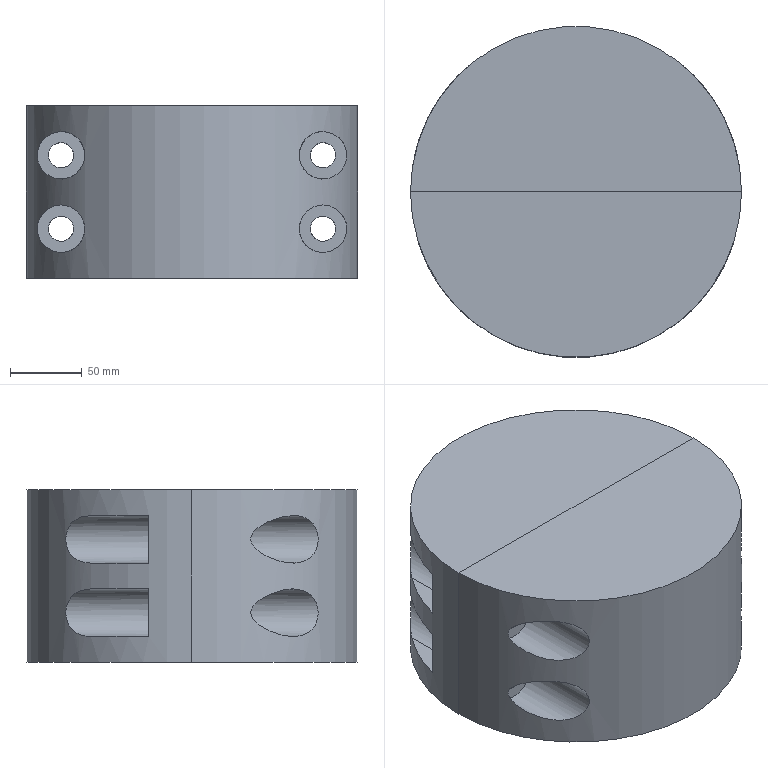Part | 2 solids | 40 faces | box 230 x 230 x 120 mm | volume 4635464 mm3 | plane 22 | cylinder 18 | commonest cylinder face diameters 33 x8 17.5 x4 21.5 x4 230 x2
STEP:
#1=CARTESIAN_POINT('',(-91.,-70.314,-69.));
#2=VERTEX_POINT('',#1);
#3=CARTESIAN_POINT('',(-96.354,-62.987,-69.619));
#4=CARTESIAN_POINT('',(-91.082,-70.404,-68.695));
#5=CARTESIAN_POINT('',(-85.319,-77.28,-69.6));
#6=CARTESIAN_POINT('',(-79.311,-83.397,-73.048));
#7=CARTESIAN_POINT('',(-75.355,-86.883,-78.919));
#8=CARTESIAN_POINT('',(-74.295,-87.779,-84.937));
#9=CARTESIAN_POINT('',(-74.785,-87.366,-89.518));
#10=CARTESIAN_POINT('',(-76.421,-85.949,-93.603));
#11=CARTESIAN_POINT('',(-79.627,-83.033,-97.936));
#12=CARTESIAN_POINT('',(-84.578,-78.089,-101.141));
#13=CARTESIAN_POINT('',(-90.444,-71.222,-102.304));
#14=CARTESIAN_POINT('',(-95.772,-63.869,-101.569));
#15=CARTESIAN_POINT('',(-99.558,-57.683,-99.78));
#16=CARTESIAN_POINT('',(-102.236,-52.713,-97.676));
#17=CARTESIAN_POINT('',(-104.052,-49.025,-95.718));
#18=CARTESIAN_POINT('',(-105.632,-45.513,-93.32));
#19=CARTESIAN_POINT('',(-106.715,-42.878,-90.795));
#20=CARTESIAN_POINT('',(-107.32,-41.324,-88.221));
#21=CARTESIAN_POINT('',(-107.546,-40.729,-86.006));
#22=CARTESIAN_POINT('',(-107.453,-40.976,-83.706));
#23=CARTESIAN_POINT('',(-106.959,-42.26,-80.962));
#24=CARTESIAN_POINT('',(-105.94,-44.789,-78.271));
#25=CARTESIAN_POINT('',(-104.42,-48.235,-75.768));
#26=CARTESIAN_POINT('',(-102.668,-51.865,-73.736));
#27=CARTESIAN_POINT('',(-100.044,-56.834,-71.521));
#28=CARTESIAN_POINT('',(-96.354,-62.987,-69.619));
#29=CARTESIAN_POINT('',(-91.082,-70.404,-68.695));
#30=CARTESIAN_POINT('',(-85.319,-77.28,-69.6));
#31=B_SPLINE_CURVE_WITH_KNOTS('',3,(#3,#4,#5,#6,#7,#8,#9,#10,#11,#12,#13,#14,#15,#16,#17,#18,#19,#20,#21,#22,#23,#24,#25,#26,#27,#28,#29,#30),.UNSPECIFIED.,.T.,.F.,(1,1,1,1,1,1,1,1,1,1,1,1,1,1,1,1,1,1,1,1,1,1,1,1,1,1,1,1,1,1,1,1),(-0.02241,-0.01793,-0.008966,0.,0.008966,0.01793,0.0269,0.03138,0.03586,0.04035,0.04483,0.05379,0.06276,0.07173,0.08069,0.08517,0.08966,0.09414,0.09862,0.1009,0.1031,0.1053,0.1076,0.1121,0.1166,0.121,0.1255,0.1345,0.1435,0.1524,0.1614,0.1703),.UNSPECIFIED.);
#32=EDGE_CURVE('',#2,#2,#31,.T.);
#33=ORIENTED_EDGE('',*,*,#32,.F.);
#34=EDGE_LOOP('',(#33));
#35=FACE_BOUND('',#34,.T.);
#36=CARTESIAN_POINT('',(-107.5,-30.,-85.5));
#37=VERTEX_POINT('',#36);
#38=CARTESIAN_POINT('',(-91.,-30.,-85.5));
#39=DIRECTION('',(0.,-1.,0.));
#40=DIRECTION('',(-1.,0.,0.));
#41=AXIS2_PLACEMENT_3D('',#38,#39,#40);
#42=CIRCLE('',#41,16.5);
#43=EDGE_CURVE('',#37,#37,#42,.T.);
#44=ORIENTED_EDGE('',*,*,#43,.F.);
#45=EDGE_LOOP('',(#44));
#46=FACE_BOUND('',#45,.T.);
#47=CARTESIAN_POINT('',(-91.,-120.,-85.5));
#48=DIRECTION('',(0.,1.,0.));
#49=DIRECTION('',(0.,0.,1.));
#50=AXIS2_PLACEMENT_3D('',#47,#48,#49);
#51=CYLINDRICAL_SURFACE('',#50,16.5);
#52=ADVANCED_FACE('',(#35,#46),#51,.F.);
#53=CARTESIAN_POINT('',(-91.,-30.,-76.75));
#54=VERTEX_POINT('',#53);
#55=CARTESIAN_POINT('',(-91.,-30.,-85.5));
#56=DIRECTION('',(0.,-1.,0.));
#57=DIRECTION('',(0.,0.,1.));
#58=AXIS2_PLACEMENT_3D('',#55,#56,#57);
#59=CIRCLE('',#58,8.75);
#60=EDGE_CURVE('',#54,#54,#59,.T.);
#61=ORIENTED_EDGE('',*,*,#60,.F.);
#62=EDGE_LOOP('',(#61));
#63=FACE_BOUND('',#62,.T.);
#64=ORIENTED_EDGE('',*,*,#43,.T.);
#65=EDGE_LOOP('',(#64));
#66=FACE_BOUND('',#65,.T.);
#67=CARTESIAN_POINT('',(-91.,-30.,-85.5));
#68=DIRECTION('',(0.,1.,0.));
#69=DIRECTION('',(0.,0.,1.));
#70=AXIS2_PLACEMENT_3D('',#67,#68,#69);
#71=PLANE('',#70);
#72=ADVANCED_FACE('',(#63,#66),#71,.F.);
#73=CARTESIAN_POINT('',(-99.75,0.,-85.5));
#74=VERTEX_POINT('',#73);
#75=CARTESIAN_POINT('',(-91.,0.,-85.5));
#76=DIRECTION('',(0.,1.,0.));
#77=DIRECTION('',(-1.,0.,0.));
#78=AXIS2_PLACEMENT_3D('',#75,#76,#77);
#79=CIRCLE('',#78,8.75);
#80=EDGE_CURVE('',#74,#74,#79,.F.);
#81=ORIENTED_EDGE('',*,*,#80,.F.);
#82=EDGE_LOOP('',(#81));
#83=FACE_BOUND('',#82,.T.);
#84=ORIENTED_EDGE('',*,*,#60,.T.);
#85=EDGE_LOOP('',(#84));
#86=FACE_BOUND('',#85,.T.);
#87=CARTESIAN_POINT('',(-91.,-120.,-85.5));
#88=DIRECTION('',(0.,1.,0.));
#89=DIRECTION('',(0.,0.,1.));
#90=AXIS2_PLACEMENT_3D('',#87,#88,#89);
#91=CYLINDRICAL_SURFACE('',#90,8.75);
#92=ADVANCED_FACE('',(#83,#86),#91,.F.);
#93=CARTESIAN_POINT('',(-91.,-30.,-43.25));
#94=VERTEX_POINT('',#93);
#95=CARTESIAN_POINT('',(-91.,-30.,-34.5));
#96=DIRECTION('',(0.,1.,0.));
#97=DIRECTION('',(0.,0.,-1.));
#98=AXIS2_PLACEMENT_3D('',#95,#96,#97);
#99=CIRCLE('',#98,8.75);
#100=EDGE_CURVE('',#94,#94,#99,.F.);
#101=ORIENTED_EDGE('',*,*,#100,.T.);
#102=EDGE_LOOP('',(#101));
#103=FACE_BOUND('',#102,.T.);
#104=CARTESIAN_POINT('',(-99.75,0.,-34.5));
#105=VERTEX_POINT('',#104);
#106=CARTESIAN_POINT('',(-91.,0.,-34.5));
#107=DIRECTION('',(0.,-1.,0.));
#108=DIRECTION('',(-1.,0.,0.));
#109=AXIS2_PLACEMENT_3D('',#106,#107,#108);
#110=CIRCLE('',#109,8.75);
#111=EDGE_CURVE('',#105,#105,#110,.T.);
#112=ORIENTED_EDGE('',*,*,#111,.F.);
#113=EDGE_LOOP('',(#112));
#114=FACE_BOUND('',#113,.T.);
#115=CARTESIAN_POINT('',(-91.,-120.,-34.5));
#116=DIRECTION('',(0.,1.,0.));
#117=DIRECTION('',(0.,0.,1.));
#118=AXIS2_PLACEMENT_3D('',#115,#116,#117);
#119=CYLINDRICAL_SURFACE('',#118,8.75);
#120=ADVANCED_FACE('',(#103,#114),#119,.F.);
#121=ORIENTED_EDGE('',*,*,#100,.F.);
#122=EDGE_LOOP('',(#121));
#123=FACE_BOUND('',#122,.T.);
#124=CARTESIAN_POINT('',(-107.5,-30.,-34.5));
#125=VERTEX_POINT('',#124);
#126=CARTESIAN_POINT('',(-91.,-30.,-34.5));
#127=DIRECTION('',(0.,1.,0.));
#128=DIRECTION('',(-1.,0.,0.));
#129=AXIS2_PLACEMENT_3D('',#126,#127,#128);
#130=CIRCLE('',#129,16.5);
#131=EDGE_CURVE('',#125,#125,#130,.T.);
#132=ORIENTED_EDGE('',*,*,#131,.F.);
#133=EDGE_LOOP('',(#132));
#134=FACE_BOUND('',#133,.T.);
#135=CARTESIAN_POINT('',(-91.,-30.,-34.5));
#136=DIRECTION('',(0.,-1.,0.));
#137=DIRECTION('',(0.,0.,-1.));
#138=AXIS2_PLACEMENT_3D('',#135,#136,#137);
#139=PLANE('',#138);
#140=ADVANCED_FACE('',(#123,#134),#139,.T.);
#141=CARTESIAN_POINT('',(-91.,-70.314,-18.));
#142=VERTEX_POINT('',#141);
#143=CARTESIAN_POINT('',(-85.296,-77.307,-18.605));
#144=CARTESIAN_POINT('',(-91.099,-70.38,-17.698));
#145=CARTESIAN_POINT('',(-95.44,-64.276,-18.453));
#146=CARTESIAN_POINT('',(-98.544,-59.334,-19.753));
#147=CARTESIAN_POINT('',(-100.712,-55.572,-21.081));
#148=CARTESIAN_POINT('',(-102.66,-51.88,-22.731));
#149=CARTESIAN_POINT('',(-104.409,-48.258,-24.752));
#150=CARTESIAN_POINT('',(-105.937,-44.797,-27.266));
#151=CARTESIAN_POINT('',(-106.953,-42.277,-29.937));
#152=CARTESIAN_POINT('',(-107.452,-40.979,-32.694));
#153=CARTESIAN_POINT('',(-107.547,-40.727,-34.996));
#154=CARTESIAN_POINT('',(-107.319,-41.327,-37.229));
#155=CARTESIAN_POINT('',(-106.714,-42.88,-39.795));
#156=CARTESIAN_POINT('',(-105.63,-45.518,-42.326));
#157=CARTESIAN_POINT('',(-104.046,-49.037,-44.723));
#158=CARTESIAN_POINT('',(-102.253,-52.679,-46.66));
#159=CARTESIAN_POINT('',(-99.557,-57.686,-48.784));
#160=CARTESIAN_POINT('',(-95.779,-63.857,-50.565));
#161=CARTESIAN_POINT('',(-90.458,-71.205,-51.304));
#162=CARTESIAN_POINT('',(-84.59,-78.077,-50.146));
#163=CARTESIAN_POINT('',(-79.635,-83.026,-46.942));
#164=CARTESIAN_POINT('',(-76.43,-85.941,-42.618));
#165=CARTESIAN_POINT('',(-74.794,-87.359,-38.545));
#166=CARTESIAN_POINT('',(-74.294,-87.779,-33.985));
#167=CARTESIAN_POINT('',(-75.338,-86.898,-27.95));
#168=CARTESIAN_POINT('',(-79.304,-83.403,-22.055));
#169=CARTESIAN_POINT('',(-85.296,-77.307,-18.605));
#170=CARTESIAN_POINT('',(-91.099,-70.38,-17.698));
#171=CARTESIAN_POINT('',(-95.44,-64.276,-18.453));
#172=B_SPLINE_CURVE_WITH_KNOTS('',3,(#143,#144,#145,#146,#147,#148,#149,#150,#151,#152,#153,#154,#155,#156,#157,#158,#159,#160,#161,#162,#163,#164,#165,#166,#167,#168,#169,#170,#171),.UNSPECIFIED.,.T.,.F.,(1,1,1,1,1,1,1,1,1,1,1,1,1,1,1,1,1,1,1,1,1,1,1,1,1,1,1,1,1,1,1,1,1),(-0.02687,-0.01791,-0.008956,0.,0.008956,0.01343,0.01791,0.02239,0.02687,0.03135,0.03583,0.03806,0.0403,0.04254,0.04478,0.04926,0.05374,0.05822,0.06269,0.07165,0.08061,0.08956,0.09852,0.103,0.1075,0.112,0.1164,0.1254,0.1343,0.1433,0.1523,0.1567,0.1612),.UNSPECIFIED.);
#173=EDGE_CURVE('',#142,#142,#172,.F.);
#174=ORIENTED_EDGE('',*,*,#173,.F.);
#175=EDGE_LOOP('',(#174));
#176=FACE_BOUND('',#175,.T.);
#177=ORIENTED_EDGE('',*,*,#131,.T.);
#178=EDGE_LOOP('',(#177));
#179=FACE_BOUND('',#178,.T.);
#180=CARTESIAN_POINT('',(-91.,-120.,-34.5));
#181=DIRECTION('',(0.,1.,0.));
#182=DIRECTION('',(0.,0.,1.));
#183=AXIS2_PLACEMENT_3D('',#180,#181,#182);
#184=CYLINDRICAL_SURFACE('',#183,16.5);
#185=ADVANCED_FACE('',(#176,#179),#184,.F.);
#186=CARTESIAN_POINT('',(91.,-30.,-43.25));
#187=VERTEX_POINT('',#186);
#188=CARTESIAN_POINT('',(91.,-30.,-34.5));
#189=DIRECTION('',(0.,-1.,0.));
#190=DIRECTION('',(0.,0.,-1.));
#191=AXIS2_PLACEMENT_3D('',#188,#189,#190);
#192=CIRCLE('',#191,8.75);
#193=EDGE_CURVE('',#187,#187,#192,.T.);
#194=ORIENTED_EDGE('',*,*,#193,.F.);
#195=EDGE_LOOP('',(#194));
#196=FACE_BOUND('',#195,.T.);
#197=CARTESIAN_POINT('',(107.5,-30.,-34.5));
#198=VERTEX_POINT('',#197);
#199=CARTESIAN_POINT('',(91.,-30.,-34.5));
#200=DIRECTION('',(0.,-1.,0.));
#201=DIRECTION('',(1.,0.,0.));
#202=AXIS2_PLACEMENT_3D('',#199,#200,#201);
#203=CIRCLE('',#202,16.5);
#204=EDGE_CURVE('',#198,#198,#203,.F.);
#205=ORIENTED_EDGE('',*,*,#204,.F.);
#206=EDGE_LOOP('',(#205));
#207=FACE_BOUND('',#206,.T.);
#208=CARTESIAN_POINT('',(91.,-30.,-34.5));
#209=DIRECTION('',(0.,-1.,0.));
#210=DIRECTION('',(0.,0.,-1.));
#211=AXIS2_PLACEMENT_3D('',#208,#209,#210);
#212=PLANE('',#211);
#213=ADVANCED_FACE('',(#196,#207),#212,.T.);
#214=CARTESIAN_POINT('',(91.,-30.,-76.75));
#215=VERTEX_POINT('',#214);
#216=CARTESIAN_POINT('',(91.,-30.,-85.5));
#217=DIRECTION('',(0.,1.,0.));
#218=DIRECTION('',(0.,0.,1.));
#219=AXIS2_PLACEMENT_3D('',#216,#217,#218);
#220=CIRCLE('',#219,8.75);
#221=EDGE_CURVE('',#215,#215,#220,.F.);
#222=ORIENTED_EDGE('',*,*,#221,.F.);
#223=EDGE_LOOP('',(#222));
#224=FACE_BOUND('',#223,.T.);
#225=CARTESIAN_POINT('',(107.5,-30.,-85.5));
#226=VERTEX_POINT('',#225);
#227=CARTESIAN_POINT('',(91.,-30.,-85.5));
#228=DIRECTION('',(0.,1.,0.));
#229=DIRECTION('',(1.,0.,0.));
#230=AXIS2_PLACEMENT_3D('',#227,#228,#229);
#231=CIRCLE('',#230,16.5);
#232=EDGE_CURVE('',#226,#226,#231,.F.);
#233=ORIENTED_EDGE('',*,*,#232,.T.);
#234=EDGE_LOOP('',(#233));
#235=FACE_BOUND('',#234,.T.);
#236=CARTESIAN_POINT('',(91.,-30.,-85.5));
#237=DIRECTION('',(0.,1.,0.));
#238=DIRECTION('',(0.,0.,1.));
#239=AXIS2_PLACEMENT_3D('',#236,#237,#238);
#240=PLANE('',#239);
#241=ADVANCED_FACE('',(#224,#235),#240,.F.);
#242=ORIENTED_EDGE('',*,*,#193,.T.);
#243=EDGE_LOOP('',(#242));
#244=FACE_BOUND('',#243,.T.);
#245=CARTESIAN_POINT('',(99.75,0.,-34.5));
#246=VERTEX_POINT('',#245);
#247=CARTESIAN_POINT('',(91.,0.,-34.5));
#248=DIRECTION('',(0.,1.,0.));
#249=DIRECTION('',(1.,0.,0.));
#250=AXIS2_PLACEMENT_3D('',#247,#248,#249);
#251=CIRCLE('',#250,8.75);
#252=EDGE_CURVE('',#246,#246,#251,.T.);
#253=ORIENTED_EDGE('',*,*,#252,.T.);
#254=EDGE_LOOP('',(#253));
#255=FACE_BOUND('',#254,.T.);
#256=CARTESIAN_POINT('',(91.,-120.,-34.5));
#257=DIRECTION('',(0.,1.,0.));
#258=DIRECTION('',(0.,0.,1.));
#259=AXIS2_PLACEMENT_3D('',#256,#257,#258);
#260=CYLINDRICAL_SURFACE('',#259,8.75);
#261=ADVANCED_FACE('',(#244,#255),#260,.F.);
#262=CARTESIAN_POINT('',(99.75,0.,-85.5));
#263=VERTEX_POINT('',#262);
#264=CARTESIAN_POINT('',(91.,0.,-85.5));
#265=DIRECTION('',(0.,-1.,0.));
#266=DIRECTION('',(1.,0.,0.));
#267=AXIS2_PLACEMENT_3D('',#264,#265,#266);
#268=CIRCLE('',#267,8.75);
#269=EDGE_CURVE('',#263,#263,#268,.T.);
#270=ORIENTED_EDGE('',*,*,#269,.F.);
#271=EDGE_LOOP('',(#270));
#272=FACE_BOUND('',#271,.T.);
#273=ORIENTED_EDGE('',*,*,#221,.T.);
#274=EDGE_LOOP('',(#273));
#275=FACE_BOUND('',#274,.T.);
#276=CARTESIAN_POINT('',(91.,-120.,-85.5));
#277=DIRECTION('',(0.,1.,0.));
#278=DIRECTION('',(0.,0.,1.));
#279=AXIS2_PLACEMENT_3D('',#276,#277,#278);
#280=CYLINDRICAL_SURFACE('',#279,8.75);
#281=ADVANCED_FACE('',(#272,#275),#280,.F.);
#282=CARTESIAN_POINT('',(91.,-70.314,-18.));
#283=VERTEX_POINT('',#282);
#284=CARTESIAN_POINT('',(85.296,-77.307,-18.605));
#285=CARTESIAN_POINT('',(91.099,-70.38,-17.698));
#286=CARTESIAN_POINT('',(95.44,-64.276,-18.453));
#287=CARTESIAN_POINT('',(98.544,-59.334,-19.753));
#288=CARTESIAN_POINT('',(100.712,-55.572,-21.081));
#289=CARTESIAN_POINT('',(102.66,-51.88,-22.731));
#290=CARTESIAN_POINT('',(104.409,-48.258,-24.752));
#291=CARTESIAN_POINT('',(105.937,-44.797,-27.266));
#292=CARTESIAN_POINT('',(106.953,-42.277,-29.937));
#293=CARTESIAN_POINT('',(107.452,-40.979,-32.694));
#294=CARTESIAN_POINT('',(107.547,-40.727,-34.996));
#295=CARTESIAN_POINT('',(107.319,-41.327,-37.229));
#296=CARTESIAN_POINT('',(106.714,-42.88,-39.795));
#297=CARTESIAN_POINT('',(105.63,-45.518,-42.326));
#298=CARTESIAN_POINT('',(104.046,-49.037,-44.723));
#299=CARTESIAN_POINT('',(102.253,-52.679,-46.66));
#300=CARTESIAN_POINT('',(99.557,-57.686,-48.784));
#301=CARTESIAN_POINT('',(95.779,-63.857,-50.565));
#302=CARTESIAN_POINT('',(90.458,-71.205,-51.304));
#303=CARTESIAN_POINT('',(84.59,-78.077,-50.146));
#304=CARTESIAN_POINT('',(79.635,-83.026,-46.942));
#305=CARTESIAN_POINT('',(76.43,-85.941,-42.618));
#306=CARTESIAN_POINT('',(74.794,-87.359,-38.545));
#307=CARTESIAN_POINT('',(74.294,-87.779,-33.985));
#308=CARTESIAN_POINT('',(75.338,-86.898,-27.95));
#309=CARTESIAN_POINT('',(79.304,-83.403,-22.055));
#310=CARTESIAN_POINT('',(85.296,-77.307,-18.605));
#311=CARTESIAN_POINT('',(91.099,-70.38,-17.698));
#312=CARTESIAN_POINT('',(95.44,-64.276,-18.453));
#313=B_SPLINE_CURVE_WITH_KNOTS('',3,(#284,#285,#286,#287,#288,#289,#290,#291,#292,#293,#294,#295,#296,#297,#298,#299,#300,#301,#302,#303,#304,#305,#306,#307,#308,#309,#310,#311,#312),.UNSPECIFIED.,.T.,.F.,(1,1,1,1,1,1,1,1,1,1,1,1,1,1,1,1,1,1,1,1,1,1,1,1,1,1,1,1,1,1,1,1,1),(-0.02687,-0.01791,-0.008956,0.,0.008956,0.01343,0.01791,0.02239,0.02687,0.03135,0.03583,0.03806,0.0403,0.04254,0.04478,0.04926,0.05374,0.05822,0.06269,0.07165,0.08061,0.08956,0.09852,0.103,0.1075,0.112,0.1164,0.1254,0.1343,0.1433,0.1523,0.1567,0.1612),.UNSPECIFIED.);
#314=EDGE_CURVE('',#283,#283,#313,.T.);
#315=ORIENTED_EDGE('',*,*,#314,.F.);
#316=EDGE_LOOP('',(#315));
#317=FACE_BOUND('',#316,.T.);
#318=ORIENTED_EDGE('',*,*,#204,.T.);
#319=EDGE_LOOP('',(#318));
#320=FACE_BOUND('',#319,.T.);
#321=CARTESIAN_POINT('',(91.,-120.,-34.5));
#322=DIRECTION('',(0.,1.,0.));
#323=DIRECTION('',(0.,0.,1.));
#324=AXIS2_PLACEMENT_3D('',#321,#322,#323);
#325=CYLINDRICAL_SURFACE('',#324,16.5);
#326=ADVANCED_FACE('',(#317,#320),#325,.F.);
#327=CARTESIAN_POINT('',(-115.,0.,-120.));
#328=VERTEX_POINT('',#327);
#329=CARTESIAN_POINT('',(115.,0.,-120.));
#330=VERTEX_POINT('',#329);
#331=CARTESIAN_POINT('',(0.,0.,-120.));
#332=DIRECTION('',(0.,0.,1.));
#333=DIRECTION('',(1.,0.,0.));
#334=AXIS2_PLACEMENT_3D('',#331,#332,#333);
#335=CIRCLE('',#334,115.);
#336=EDGE_CURVE('',#328,#330,#335,.T.);
#337=ORIENTED_EDGE('',*,*,#336,.F.);
#338=CARTESIAN_POINT('',(115.,0.,-120.));
#339=DIRECTION('',(-1.,0.,0.));
#340=VECTOR('',#339,1000.);
#341=LINE('',#338,#340);
#342=EDGE_CURVE('',#330,#328,#341,.T.);
#343=ORIENTED_EDGE('',*,*,#342,.F.);
#344=EDGE_LOOP('',(#337,#343));
#345=FACE_BOUND('',#344,.T.);
#346=CARTESIAN_POINT('',(0.,0.,-120.));
#347=DIRECTION('',(0.,0.,1.));
#348=DIRECTION('',(1.,0.,0.));
#349=AXIS2_PLACEMENT_3D('',#346,#347,#348);
#350=PLANE('',#349);
#351=ADVANCED_FACE('',(#345),#350,.F.);
#352=ORIENTED_EDGE('',*,*,#80,.T.);
#353=EDGE_LOOP('',(#352));
#354=FACE_BOUND('',#353,.T.);
#355=ORIENTED_EDGE('',*,*,#111,.T.);
#356=EDGE_LOOP('',(#355));
#357=FACE_BOUND('',#356,.T.);
#358=ORIENTED_EDGE('',*,*,#269,.T.);
#359=EDGE_LOOP('',(#358));
#360=FACE_BOUND('',#359,.T.);
#361=CARTESIAN_POINT('',(115.,0.,0.));
#362=VERTEX_POINT('',#361);
#363=CARTESIAN_POINT('',(-115.,0.,0.));
#364=VERTEX_POINT('',#363);
#365=CARTESIAN_POINT('',(115.,0.,0.));
#366=DIRECTION('',(-1.,0.,0.));
#367=VECTOR('',#366,1000.);
#368=LINE('',#365,#367);
#369=EDGE_CURVE('',#362,#364,#368,.T.);
#370=ORIENTED_EDGE('',*,*,#369,.F.);
#371=CARTESIAN_POINT('',(115.,0.,-120.));
#372=DIRECTION('',(0.,0.,1.));
#373=VECTOR('',#372,1000.);
#374=LINE('',#371,#373);
#375=EDGE_CURVE('',#330,#362,#374,.T.);
#376=ORIENTED_EDGE('',*,*,#375,.F.);
#377=ORIENTED_EDGE('',*,*,#342,.T.);
#378=CARTESIAN_POINT('',(-115.,0.,-120.));
#379=DIRECTION('',(0.,0.,1.));
#380=VECTOR('',#379,1000.);
#381=LINE('',#378,#380);
#382=EDGE_CURVE('',#364,#328,#381,.F.);
#383=ORIENTED_EDGE('',*,*,#382,.F.);
#384=EDGE_LOOP('',(#370,#376,#377,#383));
#385=FACE_BOUND('',#384,.T.);
#386=ORIENTED_EDGE('',*,*,#252,.F.);
#387=EDGE_LOOP('',(#386));
#388=FACE_BOUND('',#387,.T.);
#389=CARTESIAN_POINT('',(115.,0.,-120.));
#390=DIRECTION('',(0.,1.,0.));
#391=DIRECTION('',(0.,0.,1.));
#392=AXIS2_PLACEMENT_3D('',#389,#390,#391);
#393=PLANE('',#392);
#394=ADVANCED_FACE('',(#354,#357,#360,#385,#388),#393,.T.);
#395=CARTESIAN_POINT('',(0.,0.,0.));
#396=DIRECTION('',(0.,0.,1.));
#397=DIRECTION('',(1.,0.,0.));
#398=AXIS2_PLACEMENT_3D('',#395,#396,#397);
#399=CIRCLE('',#398,115.);
#400=EDGE_CURVE('',#364,#362,#399,.T.);
#401=ORIENTED_EDGE('',*,*,#400,.T.);
#402=ORIENTED_EDGE('',*,*,#369,.T.);
#403=EDGE_LOOP('',(#401,#402));
#404=FACE_BOUND('',#403,.T.);
#405=CARTESIAN_POINT('',(0.,0.,0.));
#406=DIRECTION('',(0.,0.,1.));
#407=DIRECTION('',(1.,0.,0.));
#408=AXIS2_PLACEMENT_3D('',#405,#406,#407);
#409=PLANE('',#408);
#410=ADVANCED_FACE('',(#404),#409,.T.);
#411=CARTESIAN_POINT('',(91.,-70.314,-69.));
#412=VERTEX_POINT('',#411);
#413=CARTESIAN_POINT('',(96.354,-62.987,-69.619));
#414=CARTESIAN_POINT('',(91.082,-70.404,-68.695));
#415=CARTESIAN_POINT('',(85.319,-77.28,-69.6));
#416=CARTESIAN_POINT('',(79.311,-83.397,-73.048));
#417=CARTESIAN_POINT('',(75.355,-86.883,-78.919));
#418=CARTESIAN_POINT('',(74.295,-87.779,-84.937));
#419=CARTESIAN_POINT('',(74.785,-87.366,-89.518));
#420=CARTESIAN_POINT('',(76.421,-85.949,-93.603));
#421=CARTESIAN_POINT('',(79.627,-83.033,-97.936));
#422=CARTESIAN_POINT('',(84.578,-78.089,-101.141));
#423=CARTESIAN_POINT('',(90.444,-71.222,-102.304));
#424=CARTESIAN_POINT('',(95.772,-63.869,-101.569));
#425=CARTESIAN_POINT('',(99.558,-57.683,-99.78));
#426=CARTESIAN_POINT('',(102.236,-52.713,-97.676));
#427=CARTESIAN_POINT('',(104.052,-49.025,-95.718));
#428=CARTESIAN_POINT('',(105.632,-45.513,-93.32));
#429=CARTESIAN_POINT('',(106.715,-42.878,-90.795));
#430=CARTESIAN_POINT('',(107.32,-41.324,-88.221));
#431=CARTESIAN_POINT('',(107.546,-40.729,-86.006));
#432=CARTESIAN_POINT('',(107.453,-40.976,-83.706));
#433=CARTESIAN_POINT('',(106.959,-42.26,-80.962));
#434=CARTESIAN_POINT('',(105.94,-44.789,-78.271));
#435=CARTESIAN_POINT('',(104.42,-48.235,-75.768));
#436=CARTESIAN_POINT('',(102.668,-51.865,-73.736));
#437=CARTESIAN_POINT('',(100.044,-56.834,-71.521));
#438=CARTESIAN_POINT('',(96.354,-62.987,-69.619));
#439=CARTESIAN_POINT('',(91.082,-70.404,-68.695));
#440=CARTESIAN_POINT('',(85.319,-77.28,-69.6));
#441=B_SPLINE_CURVE_WITH_KNOTS('',3,(#413,#414,#415,#416,#417,#418,#419,#420,#421,#422,#423,#424,#425,#426,#427,#428,#429,#430,#431,#432,#433,#434,#435,#436,#437,#438,#439,#440),.UNSPECIFIED.,.T.,.F.,(1,1,1,1,1,1,1,1,1,1,1,1,1,1,1,1,1,1,1,1,1,1,1,1,1,1,1,1,1,1,1,1),(-0.02241,-0.01793,-0.008966,0.,0.008966,0.01793,0.0269,0.03138,0.03586,0.04035,0.04483,0.05379,0.06276,0.07173,0.08069,0.08517,0.08966,0.09414,0.09862,0.1009,0.1031,0.1053,0.1076,0.1121,0.1166,0.121,0.1255,0.1345,0.1435,0.1524,0.1614,0.1703),.UNSPECIFIED.);
#442=EDGE_CURVE('',#412,#412,#441,.T.);
#443=ORIENTED_EDGE('',*,*,#442,.T.);
#444=EDGE_LOOP('',(#443));
#445=FACE_BOUND('',#444,.T.);
#446=ORIENTED_EDGE('',*,*,#232,.F.);
#447=EDGE_LOOP('',(#446));
#448=FACE_BOUND('',#447,.T.);
#449=CARTESIAN_POINT('',(91.,-120.,-85.5));
#450=DIRECTION('',(0.,1.,0.));
#451=DIRECTION('',(0.,0.,1.));
#452=AXIS2_PLACEMENT_3D('',#449,#450,#451);
#453=CYLINDRICAL_SURFACE('',#452,16.5);
#454=ADVANCED_FACE('',(#445,#448),#453,.F.);
#455=ORIENTED_EDGE('',*,*,#173,.T.);
#456=EDGE_LOOP('',(#455));
#457=FACE_BOUND('',#456,.T.);
#458=ORIENTED_EDGE('',*,*,#442,.F.);
#459=EDGE_LOOP('',(#458));
#460=FACE_BOUND('',#459,.T.);
#461=ORIENTED_EDGE('',*,*,#400,.F.);
#462=ORIENTED_EDGE('',*,*,#382,.T.);
#463=ORIENTED_EDGE('',*,*,#336,.T.);
#464=ORIENTED_EDGE('',*,*,#375,.T.);
#465=EDGE_LOOP('',(#461,#462,#463,#464));
#466=FACE_BOUND('',#465,.T.);
#467=ORIENTED_EDGE('',*,*,#314,.T.);
#468=EDGE_LOOP('',(#467));
#469=FACE_BOUND('',#468,.T.);
#470=ORIENTED_EDGE('',*,*,#32,.T.);
#471=EDGE_LOOP('',(#470));
#472=FACE_BOUND('',#471,.T.);
#473=CARTESIAN_POINT('',(0.,0.,-120.));
#474=DIRECTION('',(0.,0.,1.));
#475=DIRECTION('',(1.,0.,0.));
#476=AXIS2_PLACEMENT_3D('',#473,#474,#475);
#477=CYLINDRICAL_SURFACE('',#476,115.);
#478=ADVANCED_FACE('',(#457,#460,#466,#469,#472),#477,.T.);
#479=CLOSED_SHELL('',(#52,#72,#92,#120,#140,#185,#213,#241,#261,#281,#326,#351,#394,#410,#454,#478));
#480=MANIFOLD_SOLID_BREP('',#479);
#481=CARTESIAN_POINT('',(-111.018,30.,-69.));
#482=VERTEX_POINT('',#481);
#483=CARTESIAN_POINT('',(-91.,70.314,-69.));
#484=VERTEX_POINT('',#483);
#485=CARTESIAN_POINT('',(0.,0.,-69.));
#486=DIRECTION('',(0.,0.,1.));
#487=DIRECTION('',(1.,0.,0.));
#488=AXIS2_PLACEMENT_3D('',#485,#486,#487);
#489=CIRCLE('',#488,115.);
#490=EDGE_CURVE('',#482,#484,#489,.F.);
#491=ORIENTED_EDGE('',*,*,#490,.T.);
#492=CARTESIAN_POINT('',(-91.,30.,-69.));
#493=VERTEX_POINT('',#492);
#494=CARTESIAN_POINT('',(-91.,120.,-69.));
#495=DIRECTION('',(0.,-1.,0.));
#496=VECTOR('',#495,1000.);
#497=LINE('',#494,#496);
#498=EDGE_CURVE('',#484,#493,#497,.T.);
#499=ORIENTED_EDGE('',*,*,#498,.T.);
#500=CARTESIAN_POINT('',(-115.,30.,-69.));
#501=DIRECTION('',(1.,0.,0.));
#502=VECTOR('',#501,1000.);
#503=LINE('',#500,#502);
#504=EDGE_CURVE('',#482,#493,#503,.T.);
#505=ORIENTED_EDGE('',*,*,#504,.F.);
#506=EDGE_LOOP('',(#491,#499,#505));
#507=FACE_BOUND('',#506,.T.);
#508=CARTESIAN_POINT('',(-115.,120.,-69.));
#509=DIRECTION('',(0.,0.,1.));
#510=DIRECTION('',(-1.,0.,0.));
#511=AXIS2_PLACEMENT_3D('',#508,#509,#510);
#512=PLANE('',#511);
#513=ADVANCED_FACE('',(#507),#512,.F.);
#514=CARTESIAN_POINT('',(-91.,70.314,-102.));
#515=VERTEX_POINT('',#514);
#516=CARTESIAN_POINT('',(-111.018,30.,-102.));
#517=VERTEX_POINT('',#516);
#518=CARTESIAN_POINT('',(0.,0.,-102.));
#519=DIRECTION('',(0.,0.,-1.));
#520=DIRECTION('',(-1.,0.,0.));
#521=AXIS2_PLACEMENT_3D('',#518,#519,#520);
#522=CIRCLE('',#521,115.);
#523=EDGE_CURVE('',#515,#517,#522,.F.);
#524=ORIENTED_EDGE('',*,*,#523,.T.);
#525=CARTESIAN_POINT('',(-91.,30.,-102.));
#526=VERTEX_POINT('',#525);
#527=CARTESIAN_POINT('',(-91.,30.,-102.));
#528=DIRECTION('',(-1.,0.,0.));
#529=VECTOR('',#528,1000.);
#530=LINE('',#527,#529);
#531=EDGE_CURVE('',#526,#517,#530,.T.);
#532=ORIENTED_EDGE('',*,*,#531,.F.);
#533=CARTESIAN_POINT('',(-91.,120.,-102.));
#534=DIRECTION('',(0.,-1.,0.));
#535=VECTOR('',#534,1000.);
#536=LINE('',#533,#535);
#537=EDGE_CURVE('',#515,#526,#536,.T.);
#538=ORIENTED_EDGE('',*,*,#537,.F.);
#539=EDGE_LOOP('',(#524,#532,#538));
#540=FACE_BOUND('',#539,.T.);
#541=CARTESIAN_POINT('',(-91.,120.,-102.));
#542=DIRECTION('',(0.,0.,-1.));
#543=DIRECTION('',(1.,0.,0.));
#544=AXIS2_PLACEMENT_3D('',#541,#542,#543);
#545=PLANE('',#544);
#546=ADVANCED_FACE('',(#540),#545,.F.);
#547=CARTESIAN_POINT('',(-101.75,30.,-85.5));
#548=VERTEX_POINT('',#547);
#549=CARTESIAN_POINT('',(-91.,30.,-85.5));
#550=DIRECTION('',(0.,-1.,0.));
#551=DIRECTION('',(-1.,0.,0.));
#552=AXIS2_PLACEMENT_3D('',#549,#550,#551);
#553=CIRCLE('',#552,10.75);
#554=EDGE_CURVE('',#548,#548,#553,.F.);
#555=ORIENTED_EDGE('',*,*,#554,.T.);
#556=EDGE_LOOP('',(#555));
#557=FACE_BOUND('',#556,.T.);
#558=CARTESIAN_POINT('',(-101.75,0.,-85.5));
#559=VERTEX_POINT('',#558);
#560=CARTESIAN_POINT('',(-91.,0.,-85.5));
#561=DIRECTION('',(0.,1.,0.));
#562=DIRECTION('',(-1.,0.,0.));
#563=AXIS2_PLACEMENT_3D('',#560,#561,#562);
#564=CIRCLE('',#563,10.75);
#565=EDGE_CURVE('',#559,#559,#564,.T.);
#566=ORIENTED_EDGE('',*,*,#565,.F.);
#567=EDGE_LOOP('',(#566));
#568=FACE_BOUND('',#567,.T.);
#569=CARTESIAN_POINT('',(-91.,120.,-85.5));
#570=DIRECTION('',(0.,-1.,0.));
#571=DIRECTION('',(0.,0.,-1.));
#572=AXIS2_PLACEMENT_3D('',#569,#570,#571);
#573=CYLINDRICAL_SURFACE('',#572,10.75);
#574=ADVANCED_FACE('',(#557,#568),#573,.F.);
#575=CARTESIAN_POINT('',(-111.018,30.,-120.));
#576=DIRECTION('',(0.,0.,1.));
#577=VECTOR('',#576,1000.);
#578=LINE('',#575,#577);
#579=EDGE_CURVE('',#517,#482,#578,.T.);
#580=ORIENTED_EDGE('',*,*,#579,.T.);
#581=ORIENTED_EDGE('',*,*,#504,.T.);
#582=CARTESIAN_POINT('',(-91.,30.,-85.5));
#583=DIRECTION('',(0.,1.,0.));
#584=DIRECTION('',(-1.,0.,0.));
#585=AXIS2_PLACEMENT_3D('',#582,#583,#584);
#586=CIRCLE('',#585,16.5);
#587=EDGE_CURVE('',#493,#526,#586,.T.);
#588=ORIENTED_EDGE('',*,*,#587,.T.);
#589=ORIENTED_EDGE('',*,*,#531,.T.);
#590=EDGE_LOOP('',(#580,#581,#588,#589));
#591=FACE_BOUND('',#590,.T.);
#592=ORIENTED_EDGE('',*,*,#554,.F.);
#593=EDGE_LOOP('',(#592));
#594=FACE_BOUND('',#593,.T.);
#595=CARTESIAN_POINT('',(-91.,30.,-85.5));
#596=DIRECTION('',(0.,-1.,0.));
#597=DIRECTION('',(0.,0.,-1.));
#598=AXIS2_PLACEMENT_3D('',#595,#596,#597);
#599=PLANE('',#598);
#600=ADVANCED_FACE('',(#591,#594),#599,.F.);
#601=CARTESIAN_POINT('',(-91.,70.314,-69.));
#602=CARTESIAN_POINT('',(-89.352,72.446,-69.));
#603=CARTESIAN_POINT('',(-85.971,76.516,-69.474));
#604=CARTESIAN_POINT('',(-80.641,82.097,-72.135));
#605=CARTESIAN_POINT('',(-75.938,86.405,-77.428));
#606=CARTESIAN_POINT('',(-73.791,88.197,-85.442));
#607=CARTESIAN_POINT('',(-75.897,86.44,-93.511));
#608=CARTESIAN_POINT('',(-80.598,82.138,-98.829));
#609=CARTESIAN_POINT('',(-85.9,76.598,-101.509));
#610=CARTESIAN_POINT('',(-89.348,72.451,-102.));
#611=CARTESIAN_POINT('',(-91.,70.314,-102.));
#612=B_SPLINE_CURVE_WITH_KNOTS('',3,(#601,#602,#603,#604,#605,#606,#607,#608,#609,#610,#611),.UNSPECIFIED.,.F.,.F.,(4,1,1,1,1,1,1,1,4),(0.,0.007969,0.01594,0.02391,0.03188,0.03985,0.04782,0.05579,0.06376),.UNSPECIFIED.);
#613=EDGE_CURVE('',#515,#484,#612,.F.);
#614=ORIENTED_EDGE('',*,*,#613,.F.);
#615=ORIENTED_EDGE('',*,*,#537,.T.);
#616=ORIENTED_EDGE('',*,*,#587,.F.);
#617=ORIENTED_EDGE('',*,*,#498,.F.);
#618=EDGE_LOOP('',(#614,#615,#616,#617));
#619=FACE_BOUND('',#618,.T.);
#620=CARTESIAN_POINT('',(-91.,120.,-85.5));
#621=DIRECTION('',(0.,-1.,0.));
#622=DIRECTION('',(0.,0.,-1.));
#623=AXIS2_PLACEMENT_3D('',#620,#621,#622);
#624=CYLINDRICAL_SURFACE('',#623,16.5);
#625=ADVANCED_FACE('',(#619),#624,.F.);
#626=CARTESIAN_POINT('',(-91.,70.314,-51.));
#627=VERTEX_POINT('',#626);
#628=CARTESIAN_POINT('',(-91.,70.314,-18.));
#629=VERTEX_POINT('',#628);
#630=CARTESIAN_POINT('',(-91.,70.314,-18.));
#631=CARTESIAN_POINT('',(-89.352,72.446,-18.));
#632=CARTESIAN_POINT('',(-85.971,76.516,-18.474));
#633=CARTESIAN_POINT('',(-80.641,82.097,-21.135));
#634=CARTESIAN_POINT('',(-75.938,86.405,-26.428));
#635=CARTESIAN_POINT('',(-73.791,88.197,-34.442));
#636=CARTESIAN_POINT('',(-75.897,86.44,-42.511));
#637=CARTESIAN_POINT('',(-80.598,82.138,-47.829));
#638=CARTESIAN_POINT('',(-85.9,76.598,-50.509));
#639=CARTESIAN_POINT('',(-89.348,72.451,-51.));
#640=CARTESIAN_POINT('',(-91.,70.314,-51.));
#641=B_SPLINE_CURVE_WITH_KNOTS('',3,(#630,#631,#632,#633,#634,#635,#636,#637,#638,#639,#640),.UNSPECIFIED.,.F.,.F.,(4,1,1,1,1,1,1,1,4),(0.,0.007969,0.01594,0.02391,0.03188,0.03985,0.04782,0.05579,0.06376),.UNSPECIFIED.);
#642=EDGE_CURVE('',#627,#629,#641,.F.);
#643=ORIENTED_EDGE('',*,*,#642,.F.);
#644=CARTESIAN_POINT('',(-91.,30.,-51.));
#645=VERTEX_POINT('',#644);
#646=CARTESIAN_POINT('',(-91.,120.,-51.));
#647=DIRECTION('',(0.,-1.,0.));
#648=VECTOR('',#647,1000.);
#649=LINE('',#646,#648);
#650=EDGE_CURVE('',#627,#645,#649,.T.);
#651=ORIENTED_EDGE('',*,*,#650,.T.);
#652=CARTESIAN_POINT('',(-91.,30.,-18.));
#653=VERTEX_POINT('',#652);
#654=CARTESIAN_POINT('',(-91.,30.,-34.5));
#655=DIRECTION('',(0.,1.,0.));
#656=DIRECTION('',(-1.,0.,0.));
#657=AXIS2_PLACEMENT_3D('',#654,#655,#656);
#658=CIRCLE('',#657,16.5);
#659=EDGE_CURVE('',#653,#645,#658,.T.);
#660=ORIENTED_EDGE('',*,*,#659,.F.);
#661=CARTESIAN_POINT('',(-91.,120.,-18.));
#662=DIRECTION('',(0.,-1.,0.));
#663=VECTOR('',#662,1000.);
#664=LINE('',#661,#663);
#665=EDGE_CURVE('',#629,#653,#664,.T.);
#666=ORIENTED_EDGE('',*,*,#665,.F.);
#667=EDGE_LOOP('',(#643,#651,#660,#666));
#668=FACE_BOUND('',#667,.T.);
#669=CARTESIAN_POINT('',(-91.,120.,-34.5));
#670=DIRECTION('',(0.,-1.,0.));
#671=DIRECTION('',(0.,0.,-1.));
#672=AXIS2_PLACEMENT_3D('',#669,#670,#671);
#673=CYLINDRICAL_SURFACE('',#672,16.5);
#674=ADVANCED_FACE('',(#668),#673,.F.);
#675=CARTESIAN_POINT('',(-111.018,30.,-51.));
#676=VERTEX_POINT('',#675);
#677=CARTESIAN_POINT('',(-111.018,30.,-18.));
#678=VERTEX_POINT('',#677);
#679=CARTESIAN_POINT('',(-111.018,30.,-120.));
#680=DIRECTION('',(0.,0.,1.));
#681=VECTOR('',#680,1000.);
#682=LINE('',#679,#681);
#683=EDGE_CURVE('',#676,#678,#682,.T.);
#684=ORIENTED_EDGE('',*,*,#683,.T.);
#685=CARTESIAN_POINT('',(-115.,30.,-18.));
#686=DIRECTION('',(1.,0.,0.));
#687=VECTOR('',#686,1000.);
#688=LINE('',#685,#687);
#689=EDGE_CURVE('',#678,#653,#688,.T.);
#690=ORIENTED_EDGE('',*,*,#689,.T.);
#691=ORIENTED_EDGE('',*,*,#659,.T.);
#692=CARTESIAN_POINT('',(-91.,30.,-51.));
#693=DIRECTION('',(-1.,0.,0.));
#694=VECTOR('',#693,1000.);
#695=LINE('',#692,#694);
#696=EDGE_CURVE('',#645,#676,#695,.T.);
#697=ORIENTED_EDGE('',*,*,#696,.T.);
#698=EDGE_LOOP('',(#684,#690,#691,#697));
#699=FACE_BOUND('',#698,.T.);
#700=CARTESIAN_POINT('',(-101.75,30.,-34.5));
#701=VERTEX_POINT('',#700);
#702=CARTESIAN_POINT('',(-91.,30.,-34.5));
#703=DIRECTION('',(0.,-1.,0.));
#704=DIRECTION('',(-1.,0.,0.));
#705=AXIS2_PLACEMENT_3D('',#702,#703,#704);
#706=CIRCLE('',#705,10.75);
#707=EDGE_CURVE('',#701,#701,#706,.F.);
#708=ORIENTED_EDGE('',*,*,#707,.F.);
#709=EDGE_LOOP('',(#708));
#710=FACE_BOUND('',#709,.T.);
#711=CARTESIAN_POINT('',(-91.,30.,-34.5));
#712=DIRECTION('',(0.,-1.,0.));
#713=DIRECTION('',(0.,0.,-1.));
#714=AXIS2_PLACEMENT_3D('',#711,#712,#713);
#715=PLANE('',#714);
#716=ADVANCED_FACE('',(#699,#710),#715,.F.);
#717=ORIENTED_EDGE('',*,*,#707,.T.);
#718=EDGE_LOOP('',(#717));
#719=FACE_BOUND('',#718,.T.);
#720=CARTESIAN_POINT('',(-101.75,0.,-34.5));
#721=VERTEX_POINT('',#720);
#722=CARTESIAN_POINT('',(-91.,0.,-34.5));
#723=DIRECTION('',(0.,1.,0.));
#724=DIRECTION('',(-1.,0.,0.));
#725=AXIS2_PLACEMENT_3D('',#722,#723,#724);
#726=CIRCLE('',#725,10.75);
#727=EDGE_CURVE('',#721,#721,#726,.T.);
#728=ORIENTED_EDGE('',*,*,#727,.F.);
#729=EDGE_LOOP('',(#728));
#730=FACE_BOUND('',#729,.T.);
#731=CARTESIAN_POINT('',(-91.,120.,-34.5));
#732=DIRECTION('',(0.,-1.,0.));
#733=DIRECTION('',(0.,0.,-1.));
#734=AXIS2_PLACEMENT_3D('',#731,#732,#733);
#735=CYLINDRICAL_SURFACE('',#734,10.75);
#736=ADVANCED_FACE('',(#719,#730),#735,.F.);
#737=CARTESIAN_POINT('',(0.,0.,-51.));
#738=DIRECTION('',(0.,0.,1.));
#739=DIRECTION('',(1.,0.,0.));
#740=AXIS2_PLACEMENT_3D('',#737,#738,#739);
#741=CIRCLE('',#740,115.);
#742=EDGE_CURVE('',#676,#627,#741,.F.);
#743=ORIENTED_EDGE('',*,*,#742,.F.);
#744=ORIENTED_EDGE('',*,*,#696,.F.);
#745=ORIENTED_EDGE('',*,*,#650,.F.);
#746=EDGE_LOOP('',(#743,#744,#745));
#747=FACE_BOUND('',#746,.T.);
#748=CARTESIAN_POINT('',(-91.,120.,-51.));
#749=DIRECTION('',(0.,0.,-1.));
#750=DIRECTION('',(1.,0.,0.));
#751=AXIS2_PLACEMENT_3D('',#748,#749,#750);
#752=PLANE('',#751);
#753=ADVANCED_FACE('',(#747),#752,.F.);
#754=CARTESIAN_POINT('',(0.,0.,-18.));
#755=DIRECTION('',(0.,0.,1.));
#756=DIRECTION('',(1.,0.,0.));
#757=AXIS2_PLACEMENT_3D('',#754,#755,#756);
#758=CIRCLE('',#757,115.);
#759=EDGE_CURVE('',#678,#629,#758,.F.);
#760=ORIENTED_EDGE('',*,*,#759,.T.);
#761=ORIENTED_EDGE('',*,*,#665,.T.);
#762=ORIENTED_EDGE('',*,*,#689,.F.);
#763=EDGE_LOOP('',(#760,#761,#762));
#764=FACE_BOUND('',#763,.T.);
#765=CARTESIAN_POINT('',(-115.,120.,-18.));
#766=DIRECTION('',(0.,0.,1.));
#767=DIRECTION('',(-1.,0.,0.));
#768=AXIS2_PLACEMENT_3D('',#765,#766,#767);
#769=PLANE('',#768);
#770=ADVANCED_FACE('',(#764),#769,.F.);
#771=CARTESIAN_POINT('',(101.75,30.,-34.5));
#772=VERTEX_POINT('',#771);
#773=CARTESIAN_POINT('',(91.,30.,-34.5));
#774=DIRECTION('',(0.,1.,0.));
#775=DIRECTION('',(1.,0.,0.));
#776=AXIS2_PLACEMENT_3D('',#773,#774,#775);
#777=CIRCLE('',#776,10.75);
#778=EDGE_CURVE('',#772,#772,#777,.T.);
#779=ORIENTED_EDGE('',*,*,#778,.T.);
#780=EDGE_LOOP('',(#779));
#781=FACE_BOUND('',#780,.T.);
#782=CARTESIAN_POINT('',(101.75,0.,-34.5));
#783=VERTEX_POINT('',#782);
#784=CARTESIAN_POINT('',(91.,0.,-34.5));
#785=DIRECTION('',(0.,-1.,0.));
#786=DIRECTION('',(1.,0.,0.));
#787=AXIS2_PLACEMENT_3D('',#784,#785,#786);
#788=CIRCLE('',#787,10.75);
#789=EDGE_CURVE('',#783,#783,#788,.T.);
#790=ORIENTED_EDGE('',*,*,#789,.T.);
#791=EDGE_LOOP('',(#790));
#792=FACE_BOUND('',#791,.T.);
#793=CARTESIAN_POINT('',(91.,120.,-34.5));
#794=DIRECTION('',(0.,-1.,0.));
#795=DIRECTION('',(0.,0.,-1.));
#796=AXIS2_PLACEMENT_3D('',#793,#794,#795);
#797=CYLINDRICAL_SURFACE('',#796,10.75);
#798=ADVANCED_FACE('',(#781,#792),#797,.F.);
#799=CARTESIAN_POINT('',(101.75,30.,-85.5));
#800=VERTEX_POINT('',#799);
#801=CARTESIAN_POINT('',(91.,30.,-85.5));
#802=DIRECTION('',(0.,1.,0.));
#803=DIRECTION('',(1.,0.,0.));
#804=AXIS2_PLACEMENT_3D('',#801,#802,#803);
#805=CIRCLE('',#804,10.75);
#806=EDGE_CURVE('',#800,#800,#805,.T.);
#807=ORIENTED_EDGE('',*,*,#806,.T.);
#808=EDGE_LOOP('',(#807));
#809=FACE_BOUND('',#808,.T.);
#810=CARTESIAN_POINT('',(101.75,0.,-85.5));
#811=VERTEX_POINT('',#810);
#812=CARTESIAN_POINT('',(91.,0.,-85.5));
#813=DIRECTION('',(0.,-1.,0.));
#814=DIRECTION('',(1.,0.,0.));
#815=AXIS2_PLACEMENT_3D('',#812,#813,#814);
#816=CIRCLE('',#815,10.75);
#817=EDGE_CURVE('',#811,#811,#816,.T.);
#818=ORIENTED_EDGE('',*,*,#817,.T.);
#819=EDGE_LOOP('',(#818));
#820=FACE_BOUND('',#819,.T.);
#821=CARTESIAN_POINT('',(91.,120.,-85.5));
#822=DIRECTION('',(0.,-1.,0.));
#823=DIRECTION('',(0.,0.,-1.));
#824=AXIS2_PLACEMENT_3D('',#821,#822,#823);
#825=CYLINDRICAL_SURFACE('',#824,10.75);
#826=ADVANCED_FACE('',(#809,#820),#825,.F.);
#827=CARTESIAN_POINT('',(115.,0.,-120.));
#828=VERTEX_POINT('',#827);
#829=CARTESIAN_POINT('',(-115.,0.,-120.));
#830=VERTEX_POINT('',#829);
#831=CARTESIAN_POINT('',(0.,0.,-120.));
#832=DIRECTION('',(0.,0.,1.));
#833=DIRECTION('',(1.,0.,0.));
#834=AXIS2_PLACEMENT_3D('',#831,#832,#833);
#835=CIRCLE('',#834,115.);
#836=EDGE_CURVE('',#828,#830,#835,.T.);
#837=ORIENTED_EDGE('',*,*,#836,.F.);
#838=CARTESIAN_POINT('',(-115.,0.,-120.));
#839=DIRECTION('',(1.,0.,0.));
#840=VECTOR('',#839,1000.);
#841=LINE('',#838,#840);
#842=EDGE_CURVE('',#830,#828,#841,.T.);
#843=ORIENTED_EDGE('',*,*,#842,.F.);
#844=EDGE_LOOP('',(#837,#843));
#845=FACE_BOUND('',#844,.T.);
#846=CARTESIAN_POINT('',(0.,0.,-120.));
#847=DIRECTION('',(0.,0.,1.));
#848=DIRECTION('',(1.,0.,0.));
#849=AXIS2_PLACEMENT_3D('',#846,#847,#848);
#850=PLANE('',#849);
#851=ADVANCED_FACE('',(#845),#850,.F.);
#852=ORIENTED_EDGE('',*,*,#727,.T.);
#853=EDGE_LOOP('',(#852));
#854=FACE_BOUND('',#853,.T.);
#855=ORIENTED_EDGE('',*,*,#565,.T.);
#856=EDGE_LOOP('',(#855));
#857=FACE_BOUND('',#856,.T.);
#858=ORIENTED_EDGE('',*,*,#817,.F.);
#859=EDGE_LOOP('',(#858));
#860=FACE_BOUND('',#859,.T.);
#861=ORIENTED_EDGE('',*,*,#789,.F.);
#862=EDGE_LOOP('',(#861));
#863=FACE_BOUND('',#862,.T.);
#864=CARTESIAN_POINT('',(-115.,0.,0.));
#865=VERTEX_POINT('',#864);
#866=CARTESIAN_POINT('',(115.,0.,0.));
#867=VERTEX_POINT('',#866);
#868=CARTESIAN_POINT('',(-115.,0.,0.));
#869=DIRECTION('',(1.,0.,0.));
#870=VECTOR('',#869,1000.);
#871=LINE('',#868,#870);
#872=EDGE_CURVE('',#865,#867,#871,.T.);
#873=ORIENTED_EDGE('',*,*,#872,.F.);
#874=CARTESIAN_POINT('',(-115.,0.,-120.));
#875=DIRECTION('',(0.,0.,1.));
#876=VECTOR('',#875,1000.);
#877=LINE('',#874,#876);
#878=EDGE_CURVE('',#830,#865,#877,.T.);
#879=ORIENTED_EDGE('',*,*,#878,.F.);
#880=ORIENTED_EDGE('',*,*,#842,.T.);
#881=CARTESIAN_POINT('',(115.,0.,-120.));
#882=DIRECTION('',(0.,0.,1.));
#883=VECTOR('',#882,1000.);
#884=LINE('',#881,#883);
#885=EDGE_CURVE('',#867,#828,#884,.F.);
#886=ORIENTED_EDGE('',*,*,#885,.F.);
#887=EDGE_LOOP('',(#873,#879,#880,#886));
#888=FACE_BOUND('',#887,.T.);
#889=CARTESIAN_POINT('',(-115.,0.,-120.));
#890=DIRECTION('',(0.,-1.,0.));
#891=DIRECTION('',(0.,0.,-1.));
#892=AXIS2_PLACEMENT_3D('',#889,#890,#891);
#893=PLANE('',#892);
#894=ADVANCED_FACE('',(#854,#857,#860,#863,#888),#893,.T.);
#895=CARTESIAN_POINT('',(0.,0.,0.));
#896=DIRECTION('',(0.,0.,1.));
#897=DIRECTION('',(1.,0.,0.));
#898=AXIS2_PLACEMENT_3D('',#895,#896,#897);
#899=CIRCLE('',#898,115.);
#900=EDGE_CURVE('',#867,#865,#899,.T.);
#901=ORIENTED_EDGE('',*,*,#900,.T.);
#902=ORIENTED_EDGE('',*,*,#872,.T.);
#903=EDGE_LOOP('',(#901,#902));
#904=FACE_BOUND('',#903,.T.);
#905=CARTESIAN_POINT('',(0.,0.,0.));
#906=DIRECTION('',(0.,0.,1.));
#907=DIRECTION('',(1.,0.,0.));
#908=AXIS2_PLACEMENT_3D('',#905,#906,#907);
#909=PLANE('',#908);
#910=ADVANCED_FACE('',(#904),#909,.T.);
#911=CARTESIAN_POINT('',(91.,70.314,-18.));
#912=VERTEX_POINT('',#911);
#913=CARTESIAN_POINT('',(111.018,30.,-18.));
#914=VERTEX_POINT('',#913);
#915=CARTESIAN_POINT('',(0.,0.,-18.));
#916=DIRECTION('',(0.,0.,1.));
#917=DIRECTION('',(1.,0.,0.));
#918=AXIS2_PLACEMENT_3D('',#915,#916,#917);
#919=CIRCLE('',#918,115.);
#920=EDGE_CURVE('',#912,#914,#919,.F.);
#921=ORIENTED_EDGE('',*,*,#920,.T.);
#922=CARTESIAN_POINT('',(91.,30.,-18.));
#923=VERTEX_POINT('',#922);
#924=CARTESIAN_POINT('',(115.,30.,-18.));
#925=DIRECTION('',(-1.,0.,0.));
#926=VECTOR('',#925,1000.);
#927=LINE('',#924,#926);
#928=EDGE_CURVE('',#923,#914,#927,.F.);
#929=ORIENTED_EDGE('',*,*,#928,.F.);
#930=CARTESIAN_POINT('',(91.,120.,-18.));
#931=DIRECTION('',(0.,-1.,0.));
#932=VECTOR('',#931,1000.);
#933=LINE('',#930,#932);
#934=EDGE_CURVE('',#923,#912,#933,.F.);
#935=ORIENTED_EDGE('',*,*,#934,.T.);
#936=EDGE_LOOP('',(#921,#929,#935));
#937=FACE_BOUND('',#936,.T.);
#938=CARTESIAN_POINT('',(115.,120.,-18.));
#939=DIRECTION('',(0.,0.,1.));
#940=DIRECTION('',(1.,0.,0.));
#941=AXIS2_PLACEMENT_3D('',#938,#939,#940);
#942=PLANE('',#941);
#943=ADVANCED_FACE('',(#937),#942,.F.);
#944=CARTESIAN_POINT('',(111.018,30.,-51.));
#945=VERTEX_POINT('',#944);
#946=CARTESIAN_POINT('',(111.018,30.,-120.));
#947=DIRECTION('',(0.,0.,1.));
#948=VECTOR('',#947,1000.);
#949=LINE('',#946,#948);
#950=EDGE_CURVE('',#914,#945,#949,.F.);
#951=ORIENTED_EDGE('',*,*,#950,.T.);
#952=CARTESIAN_POINT('',(91.,30.,-51.));
#953=VERTEX_POINT('',#952);
#954=CARTESIAN_POINT('',(91.,30.,-51.));
#955=DIRECTION('',(1.,0.,0.));
#956=VECTOR('',#955,1000.);
#957=LINE('',#954,#956);
#958=EDGE_CURVE('',#945,#953,#957,.F.);
#959=ORIENTED_EDGE('',*,*,#958,.T.);
#960=CARTESIAN_POINT('',(91.,30.,-34.5));
#961=DIRECTION('',(0.,-1.,0.));
#962=DIRECTION('',(1.,0.,0.));
#963=AXIS2_PLACEMENT_3D('',#960,#961,#962);
#964=CIRCLE('',#963,16.5);
#965=EDGE_CURVE('',#953,#923,#964,.F.);
#966=ORIENTED_EDGE('',*,*,#965,.T.);
#967=ORIENTED_EDGE('',*,*,#928,.T.);
#968=EDGE_LOOP('',(#951,#959,#966,#967));
#969=FACE_BOUND('',#968,.T.);
#970=ORIENTED_EDGE('',*,*,#778,.F.);
#971=EDGE_LOOP('',(#970));
#972=FACE_BOUND('',#971,.T.);
#973=CARTESIAN_POINT('',(91.,30.,-34.5));
#974=DIRECTION('',(0.,-1.,0.));
#975=DIRECTION('',(0.,0.,-1.));
#976=AXIS2_PLACEMENT_3D('',#973,#974,#975);
#977=PLANE('',#976);
#978=ADVANCED_FACE('',(#969,#972),#977,.F.);
#979=CARTESIAN_POINT('',(91.,70.314,-51.));
#980=VERTEX_POINT('',#979);
#981=CARTESIAN_POINT('',(0.,0.,-51.));
#982=DIRECTION('',(0.,0.,-1.));
#983=DIRECTION('',(-1.,0.,0.));
#984=AXIS2_PLACEMENT_3D('',#981,#982,#983);
#985=CIRCLE('',#984,115.);
#986=EDGE_CURVE('',#945,#980,#985,.F.);
#987=ORIENTED_EDGE('',*,*,#986,.T.);
#988=CARTESIAN_POINT('',(91.,120.,-51.));
#989=DIRECTION('',(0.,-1.,0.));
#990=VECTOR('',#989,1000.);
#991=LINE('',#988,#990);
#992=EDGE_CURVE('',#953,#980,#991,.F.);
#993=ORIENTED_EDGE('',*,*,#992,.F.);
#994=ORIENTED_EDGE('',*,*,#958,.F.);
#995=EDGE_LOOP('',(#987,#993,#994));
#996=FACE_BOUND('',#995,.T.);
#997=CARTESIAN_POINT('',(91.,120.,-51.));
#998=DIRECTION('',(0.,0.,-1.));
#999=DIRECTION('',(-1.,0.,0.));
#1000=AXIS2_PLACEMENT_3D('',#997,#998,#999);
#1001=PLANE('',#1000);
#1002=ADVANCED_FACE('',(#996),#1001,.F.);
#1003=CARTESIAN_POINT('',(91.,70.314,-51.));
#1004=CARTESIAN_POINT('',(89.352,72.446,-51.));
#1005=CARTESIAN_POINT('',(85.971,76.516,-50.526));
#1006=CARTESIAN_POINT('',(80.641,82.097,-47.865));
#1007=CARTESIAN_POINT('',(75.938,86.405,-42.572));
#1008=CARTESIAN_POINT('',(73.791,88.197,-34.558));
#1009=CARTESIAN_POINT('',(75.897,86.44,-26.489));
#1010=CARTESIAN_POINT('',(80.598,82.138,-21.171));
#1011=CARTESIAN_POINT('',(85.9,76.598,-18.491));
#1012=CARTESIAN_POINT('',(89.348,72.451,-18.));
#1013=CARTESIAN_POINT('',(91.,70.314,-18.));
#1014=B_SPLINE_CURVE_WITH_KNOTS('',3,(#1003,#1004,#1005,#1006,#1007,#1008,#1009,#1010,#1011,#1012,#1013),.UNSPECIFIED.,.F.,.F.,(4,1,1,1,1,1,1,1,4),(0.,0.007969,0.01594,0.02391,0.03188,0.03985,0.04782,0.05579,0.06376),.UNSPECIFIED.);
#1015=EDGE_CURVE('',#980,#912,#1014,.T.);
#1016=ORIENTED_EDGE('',*,*,#1015,.T.);
#1017=ORIENTED_EDGE('',*,*,#934,.F.);
#1018=ORIENTED_EDGE('',*,*,#965,.F.);
#1019=ORIENTED_EDGE('',*,*,#992,.T.);
#1020=EDGE_LOOP('',(#1016,#1017,#1018,#1019));
#1021=FACE_BOUND('',#1020,.T.);
#1022=CARTESIAN_POINT('',(91.,120.,-34.5));
#1023=DIRECTION('',(0.,-1.,0.));
#1024=DIRECTION('',(0.,0.,-1.));
#1025=AXIS2_PLACEMENT_3D('',#1022,#1023,#1024);
#1026=CYLINDRICAL_SURFACE('',#1025,16.5);
#1027=ADVANCED_FACE('',(#1021),#1026,.F.);
#1028=CARTESIAN_POINT('',(91.,70.314,-69.));
#1029=VERTEX_POINT('',#1028);
#1030=CARTESIAN_POINT('',(111.018,30.,-69.));
#1031=VERTEX_POINT('',#1030);
#1032=CARTESIAN_POINT('',(0.,0.,-69.));
#1033=DIRECTION('',(0.,0.,1.));
#1034=DIRECTION('',(1.,0.,0.));
#1035=AXIS2_PLACEMENT_3D('',#1032,#1033,#1034);
#1036=CIRCLE('',#1035,115.);
#1037=EDGE_CURVE('',#1029,#1031,#1036,.F.);
#1038=ORIENTED_EDGE('',*,*,#1037,.T.);
#1039=CARTESIAN_POINT('',(91.,30.,-69.));
#1040=VERTEX_POINT('',#1039);
#1041=CARTESIAN_POINT('',(115.,30.,-69.));
#1042=DIRECTION('',(-1.,0.,0.));
#1043=VECTOR('',#1042,1000.);
#1044=LINE('',#1041,#1043);
#1045=EDGE_CURVE('',#1040,#1031,#1044,.F.);
#1046=ORIENTED_EDGE('',*,*,#1045,.F.);
#1047=CARTESIAN_POINT('',(91.,120.,-69.));
#1048=DIRECTION('',(0.,-1.,0.));
#1049=VECTOR('',#1048,1000.);
#1050=LINE('',#1047,#1049);
#1051=EDGE_CURVE('',#1040,#1029,#1050,.F.);
#1052=ORIENTED_EDGE('',*,*,#1051,.T.);
#1053=EDGE_LOOP('',(#1038,#1046,#1052));
#1054=FACE_BOUND('',#1053,.T.);
#1055=CARTESIAN_POINT('',(115.,120.,-69.));
#1056=DIRECTION('',(0.,0.,1.));
#1057=DIRECTION('',(1.,0.,0.));
#1058=AXIS2_PLACEMENT_3D('',#1055,#1056,#1057);
#1059=PLANE('',#1058);
#1060=ADVANCED_FACE('',(#1054),#1059,.F.);
#1061=CARTESIAN_POINT('',(111.018,30.,-102.));
#1062=VERTEX_POINT('',#1061);
#1063=CARTESIAN_POINT('',(111.018,30.,-120.));
#1064=DIRECTION('',(0.,0.,1.));
#1065=VECTOR('',#1064,1000.);
#1066=LINE('',#1063,#1065);
#1067=EDGE_CURVE('',#1031,#1062,#1066,.F.);
#1068=ORIENTED_EDGE('',*,*,#1067,.T.);
#1069=CARTESIAN_POINT('',(91.,30.,-102.));
#1070=VERTEX_POINT('',#1069);
#1071=CARTESIAN_POINT('',(91.,30.,-102.));
#1072=DIRECTION('',(1.,0.,0.));
#1073=VECTOR('',#1072,1000.);
#1074=LINE('',#1071,#1073);
#1075=EDGE_CURVE('',#1062,#1070,#1074,.F.);
#1076=ORIENTED_EDGE('',*,*,#1075,.T.);
#1077=CARTESIAN_POINT('',(91.,30.,-85.5));
#1078=DIRECTION('',(0.,-1.,0.));
#1079=DIRECTION('',(1.,0.,0.));
#1080=AXIS2_PLACEMENT_3D('',#1077,#1078,#1079);
#1081=CIRCLE('',#1080,16.5);
#1082=EDGE_CURVE('',#1070,#1040,#1081,.F.);
#1083=ORIENTED_EDGE('',*,*,#1082,.T.);
#1084=ORIENTED_EDGE('',*,*,#1045,.T.);
#1085=EDGE_LOOP('',(#1068,#1076,#1083,#1084));
#1086=FACE_BOUND('',#1085,.T.);
#1087=ORIENTED_EDGE('',*,*,#806,.F.);
#1088=EDGE_LOOP('',(#1087));
#1089=FACE_BOUND('',#1088,.T.);
#1090=CARTESIAN_POINT('',(91.,30.,-85.5));
#1091=DIRECTION('',(0.,-1.,0.));
#1092=DIRECTION('',(0.,0.,-1.));
#1093=AXIS2_PLACEMENT_3D('',#1090,#1091,#1092);
#1094=PLANE('',#1093);
#1095=ADVANCED_FACE('',(#1086,#1089),#1094,.F.);
#1096=CARTESIAN_POINT('',(91.,70.314,-102.));
#1097=VERTEX_POINT('',#1096);
#1098=CARTESIAN_POINT('',(0.,0.,-102.));
#1099=DIRECTION('',(0.,0.,-1.));
#1100=DIRECTION('',(-1.,0.,0.));
#1101=AXIS2_PLACEMENT_3D('',#1098,#1099,#1100);
#1102=CIRCLE('',#1101,115.);
#1103=EDGE_CURVE('',#1062,#1097,#1102,.F.);
#1104=ORIENTED_EDGE('',*,*,#1103,.T.);
#1105=CARTESIAN_POINT('',(91.,120.,-102.));
#1106=DIRECTION('',(0.,-1.,0.));
#1107=VECTOR('',#1106,1000.);
#1108=LINE('',#1105,#1107);
#1109=EDGE_CURVE('',#1070,#1097,#1108,.F.);
#1110=ORIENTED_EDGE('',*,*,#1109,.F.);
#1111=ORIENTED_EDGE('',*,*,#1075,.F.);
#1112=EDGE_LOOP('',(#1104,#1110,#1111));
#1113=FACE_BOUND('',#1112,.T.);
#1114=CARTESIAN_POINT('',(91.,120.,-102.));
#1115=DIRECTION('',(0.,0.,-1.));
#1116=DIRECTION('',(-1.,0.,0.));
#1117=AXIS2_PLACEMENT_3D('',#1114,#1115,#1116);
#1118=PLANE('',#1117);
#1119=ADVANCED_FACE('',(#1113),#1118,.F.);
#1120=CARTESIAN_POINT('',(91.,70.314,-102.));
#1121=CARTESIAN_POINT('',(89.352,72.446,-102.));
#1122=CARTESIAN_POINT('',(85.971,76.516,-101.526));
#1123=CARTESIAN_POINT('',(80.641,82.097,-98.865));
#1124=CARTESIAN_POINT('',(75.938,86.405,-93.572));
#1125=CARTESIAN_POINT('',(73.791,88.197,-85.558));
#1126=CARTESIAN_POINT('',(75.897,86.44,-77.489));
#1127=CARTESIAN_POINT('',(80.598,82.138,-72.171));
#1128=CARTESIAN_POINT('',(85.9,76.598,-69.491));
#1129=CARTESIAN_POINT('',(89.348,72.451,-69.));
#1130=CARTESIAN_POINT('',(91.,70.314,-69.));
#1131=B_SPLINE_CURVE_WITH_KNOTS('',3,(#1120,#1121,#1122,#1123,#1124,#1125,#1126,#1127,#1128,#1129,#1130),.UNSPECIFIED.,.F.,.F.,(4,1,1,1,1,1,1,1,4),(0.,0.007969,0.01594,0.02391,0.03188,0.03985,0.04782,0.05579,0.06376),.UNSPECIFIED.);
#1132=EDGE_CURVE('',#1097,#1029,#1131,.T.);
#1133=ORIENTED_EDGE('',*,*,#1132,.T.);
#1134=ORIENTED_EDGE('',*,*,#1051,.F.);
#1135=ORIENTED_EDGE('',*,*,#1082,.F.);
#1136=ORIENTED_EDGE('',*,*,#1109,.T.);
#1137=EDGE_LOOP('',(#1133,#1134,#1135,#1136));
#1138=FACE_BOUND('',#1137,.T.);
#1139=CARTESIAN_POINT('',(91.,120.,-85.5));
#1140=DIRECTION('',(0.,-1.,0.));
#1141=DIRECTION('',(0.,0.,-1.));
#1142=AXIS2_PLACEMENT_3D('',#1139,#1140,#1141);
#1143=CYLINDRICAL_SURFACE('',#1142,16.5);
#1144=ADVANCED_FACE('',(#1138),#1143,.F.);
#1145=ORIENTED_EDGE('',*,*,#1132,.F.);
#1146=ORIENTED_EDGE('',*,*,#1103,.F.);
#1147=ORIENTED_EDGE('',*,*,#1067,.F.);
#1148=ORIENTED_EDGE('',*,*,#1037,.F.);
#1149=EDGE_LOOP('',(#1145,#1146,#1147,#1148));
#1150=FACE_BOUND('',#1149,.T.);
#1151=ORIENTED_EDGE('',*,*,#1015,.F.);
#1152=ORIENTED_EDGE('',*,*,#986,.F.);
#1153=ORIENTED_EDGE('',*,*,#950,.F.);
#1154=ORIENTED_EDGE('',*,*,#920,.F.);
#1155=EDGE_LOOP('',(#1151,#1152,#1153,#1154));
#1156=FACE_BOUND('',#1155,.T.);
#1157=ORIENTED_EDGE('',*,*,#900,.F.);
#1158=ORIENTED_EDGE('',*,*,#885,.T.);
#1159=ORIENTED_EDGE('',*,*,#836,.T.);
#1160=ORIENTED_EDGE('',*,*,#878,.T.);
#1161=EDGE_LOOP('',(#1157,#1158,#1159,#1160));
#1162=FACE_BOUND('',#1161,.T.);
#1163=ORIENTED_EDGE('',*,*,#490,.F.);
#1164=ORIENTED_EDGE('',*,*,#579,.F.);
#1165=ORIENTED_EDGE('',*,*,#523,.F.);
#1166=ORIENTED_EDGE('',*,*,#613,.T.);
#1167=EDGE_LOOP('',(#1163,#1164,#1165,#1166));
#1168=FACE_BOUND('',#1167,.T.);
#1169=ORIENTED_EDGE('',*,*,#683,.F.);
#1170=ORIENTED_EDGE('',*,*,#742,.T.);
#1171=ORIENTED_EDGE('',*,*,#642,.T.);
#1172=ORIENTED_EDGE('',*,*,#759,.F.);
#1173=EDGE_LOOP('',(#1169,#1170,#1171,#1172));
#1174=FACE_BOUND('',#1173,.T.);
#1175=CARTESIAN_POINT('',(0.,0.,-120.));
#1176=DIRECTION('',(0.,0.,1.));
#1177=DIRECTION('',(1.,0.,0.));
#1178=AXIS2_PLACEMENT_3D('',#1175,#1176,#1177);
#1179=CYLINDRICAL_SURFACE('',#1178,115.);
#1180=ADVANCED_FACE('',(#1150,#1156,#1162,#1168,#1174),#1179,.T.);
#1181=CLOSED_SHELL('',(#513,#546,#574,#600,#625,#674,#716,#736,#753,#770,#798,#826,#851,#894,#910,#943,#978,#1002,#1027,#1060,#1095,#1119,#1144,#1180));
#1182=MANIFOLD_SOLID_BREP('',#1181);
#1183=(LENGTH_UNIT()NAMED_UNIT(*)SI_UNIT(.MILLI.,.METRE.));
#1184=UNCERTAINTY_MEASURE_WITH_UNIT(LENGTH_MEASURE(0.0508),#1183,'','');
#1185=(NAMED_UNIT(*)PLANE_ANGLE_UNIT()SI_UNIT($,.RADIAN.));
#1186=(NAMED_UNIT(*)SI_UNIT($,.STERADIAN.)SOLID_ANGLE_UNIT());
#1187=(GEOMETRIC_REPRESENTATION_CONTEXT(3)GLOBAL_UNCERTAINTY_ASSIGNED_CONTEXT((#1184))GLOBAL_UNIT_ASSIGNED_CONTEXT((#1183,#1185,#1186))REPRESENTATION_CONTEXT('',''));
#1188=ADVANCED_BREP_SHAPE_REPRESENTATION('',(#480,#1182),#1187);